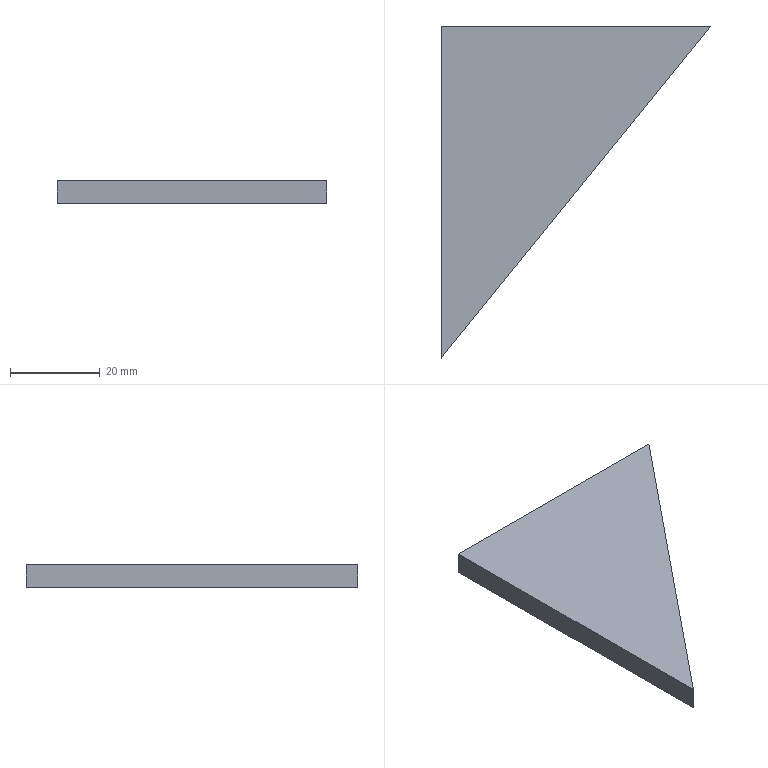Part | STEP file | Guide wheel mechanism revised.sldasm-Part-358 | 1 solid | 5 faces | box 60 x 74 x 5 mm | volume 11100 mm3 | plane 5
STEP:
#1=CARTESIAN_POINT('',(180.,74.,55.));
#2=VERTEX_POINT('',#1);
#3=CARTESIAN_POINT('',(120.,74.,55.));
#4=VERTEX_POINT('',#3);
#5=CARTESIAN_POINT('',(120.,74.,55.));
#6=DIRECTION('',(-1.,0.,0.));
#7=VECTOR('',#6,1000.);
#8=LINE('',#5,#7);
#9=EDGE_CURVE('',#2,#4,#8,.T.);
#10=ORIENTED_EDGE('',*,*,#9,.F.);
#11=CARTESIAN_POINT('',(180.,74.,50.));
#12=VERTEX_POINT('',#11);
#13=CARTESIAN_POINT('',(180.,74.,50.));
#14=DIRECTION('',(0.,0.,1.));
#15=VECTOR('',#14,1000.);
#16=LINE('',#13,#15);
#17=EDGE_CURVE('',#12,#2,#16,.T.);
#18=ORIENTED_EDGE('',*,*,#17,.F.);
#19=CARTESIAN_POINT('',(120.,74.,50.));
#20=VERTEX_POINT('',#19);
#21=CARTESIAN_POINT('',(120.,74.,50.));
#22=DIRECTION('',(-1.,0.,0.));
#23=VECTOR('',#22,1000.);
#24=LINE('',#21,#23);
#25=EDGE_CURVE('',#12,#20,#24,.T.);
#26=ORIENTED_EDGE('',*,*,#25,.T.);
#27=CARTESIAN_POINT('',(120.,74.,50.));
#28=DIRECTION('',(0.,0.,1.));
#29=VECTOR('',#28,1000.);
#30=LINE('',#27,#29);
#31=EDGE_CURVE('',#20,#4,#30,.T.);
#32=ORIENTED_EDGE('',*,*,#31,.T.);
#33=EDGE_LOOP('',(#10,#18,#26,#32));
#34=FACE_OUTER_BOUND('',#33,.T.);
#35=CARTESIAN_POINT('',(120.,74.,50.));
#36=DIRECTION('',(0.,1.,0.));
#37=DIRECTION('',(0.,0.,1.));
#38=AXIS2_PLACEMENT_3D('',#35,#36,#37);
#39=PLANE('',#38);
#40=ADVANCED_FACE('',(#34),#39,.T.);
#41=CARTESIAN_POINT('',(120.,0.,55.));
#42=VERTEX_POINT('',#41);
#43=CARTESIAN_POINT('',(180.,74.,55.));
#44=DIRECTION('',(0.6298,0.7768,0.));
#45=VECTOR('',#44,1000.);
#46=LINE('',#43,#45);
#47=EDGE_CURVE('',#42,#2,#46,.T.);
#48=ORIENTED_EDGE('',*,*,#47,.F.);
#49=CARTESIAN_POINT('',(120.,0.,50.));
#50=VERTEX_POINT('',#49);
#51=CARTESIAN_POINT('',(120.,0.,50.));
#52=DIRECTION('',(0.,0.,1.));
#53=VECTOR('',#52,1000.);
#54=LINE('',#51,#53);
#55=EDGE_CURVE('',#50,#42,#54,.T.);
#56=ORIENTED_EDGE('',*,*,#55,.F.);
#57=CARTESIAN_POINT('',(180.,74.,50.));
#58=DIRECTION('',(0.6298,0.7768,0.));
#59=VECTOR('',#58,1000.);
#60=LINE('',#57,#59);
#61=EDGE_CURVE('',#50,#12,#60,.T.);
#62=ORIENTED_EDGE('',*,*,#61,.T.);
#63=ORIENTED_EDGE('',*,*,#17,.T.);
#64=EDGE_LOOP('',(#48,#56,#62,#63));
#65=FACE_OUTER_BOUND('',#64,.T.);
#66=CARTESIAN_POINT('',(180.,74.,50.));
#67=DIRECTION('',(0.7768,-0.6298,0.));
#68=DIRECTION('',(0.6298,0.7768,0.));
#69=AXIS2_PLACEMENT_3D('',#66,#67,#68);
#70=PLANE('',#69);
#71=ADVANCED_FACE('',(#65),#70,.T.);
#72=CARTESIAN_POINT('',(120.,0.,55.));
#73=DIRECTION('',(0.,-1.,0.));
#74=VECTOR('',#73,1000.);
#75=LINE('',#72,#74);
#76=EDGE_CURVE('',#4,#42,#75,.T.);
#77=ORIENTED_EDGE('',*,*,#76,.F.);
#78=ORIENTED_EDGE('',*,*,#31,.F.);
#79=CARTESIAN_POINT('',(120.,0.,50.));
#80=DIRECTION('',(0.,-1.,0.));
#81=VECTOR('',#80,1000.);
#82=LINE('',#79,#81);
#83=EDGE_CURVE('',#20,#50,#82,.T.);
#84=ORIENTED_EDGE('',*,*,#83,.T.);
#85=ORIENTED_EDGE('',*,*,#55,.T.);
#86=EDGE_LOOP('',(#77,#78,#84,#85));
#87=FACE_OUTER_BOUND('',#86,.T.);
#88=CARTESIAN_POINT('',(120.,0.,50.));
#89=DIRECTION('',(-1.,0.,0.));
#90=DIRECTION('',(0.,0.,1.));
#91=AXIS2_PLACEMENT_3D('',#88,#89,#90);
#92=PLANE('',#91);
#93=ADVANCED_FACE('',(#87),#92,.T.);
#94=ORIENTED_EDGE('',*,*,#25,.F.);
#95=ORIENTED_EDGE('',*,*,#61,.F.);
#96=ORIENTED_EDGE('',*,*,#83,.F.);
#97=EDGE_LOOP('',(#94,#95,#96));
#98=FACE_OUTER_BOUND('',#97,.T.);
#99=CARTESIAN_POINT('',(0.,0.,50.));
#100=DIRECTION('',(0.,0.,1.));
#101=DIRECTION('',(1.,0.,0.));
#102=AXIS2_PLACEMENT_3D('',#99,#100,#101);
#103=PLANE('',#102);
#104=ADVANCED_FACE('',(#98),#103,.F.);
#105=ORIENTED_EDGE('',*,*,#9,.T.);
#106=ORIENTED_EDGE('',*,*,#76,.T.);
#107=ORIENTED_EDGE('',*,*,#47,.T.);
#108=EDGE_LOOP('',(#105,#106,#107));
#109=FACE_OUTER_BOUND('',#108,.T.);
#110=CARTESIAN_POINT('',(0.,0.,55.));
#111=DIRECTION('',(0.,0.,1.));
#112=DIRECTION('',(1.,0.,0.));
#113=AXIS2_PLACEMENT_3D('',#110,#111,#112);
#114=PLANE('',#113);
#115=ADVANCED_FACE('',(#109),#114,.T.);
#116=CLOSED_SHELL('',(#40,#71,#93,#104,#115));
#117=MANIFOLD_SOLID_BREP('',#116);
#118=CARTESIAN_POINT('',(0.,0.,0.));
#119=DIRECTION('',(0.,0.,1.));
#120=DIRECTION('',(1.,0.,0.));
#121=AXIS2_PLACEMENT_3D('',#118,#119,#120);
#122=(LENGTH_UNIT()NAMED_UNIT(*)SI_UNIT(.MILLI.,.METRE.));
#123=UNCERTAINTY_MEASURE_WITH_UNIT(LENGTH_MEASURE(0.00001),#122,'','');
#124=(NAMED_UNIT(*)PLANE_ANGLE_UNIT()SI_UNIT($,.RADIAN.));
#125=(NAMED_UNIT(*)SI_UNIT($,.STERADIAN.)SOLID_ANGLE_UNIT());
#126=(GEOMETRIC_REPRESENTATION_CONTEXT(3)GLOBAL_UNCERTAINTY_ASSIGNED_CONTEXT((#123))GLOBAL_UNIT_ASSIGNED_CONTEXT((#122,#124,#125))REPRESENTATION_CONTEXT('',''));
#127=ADVANCED_BREP_SHAPE_REPRESENTATION('',(#117,#121),#126);